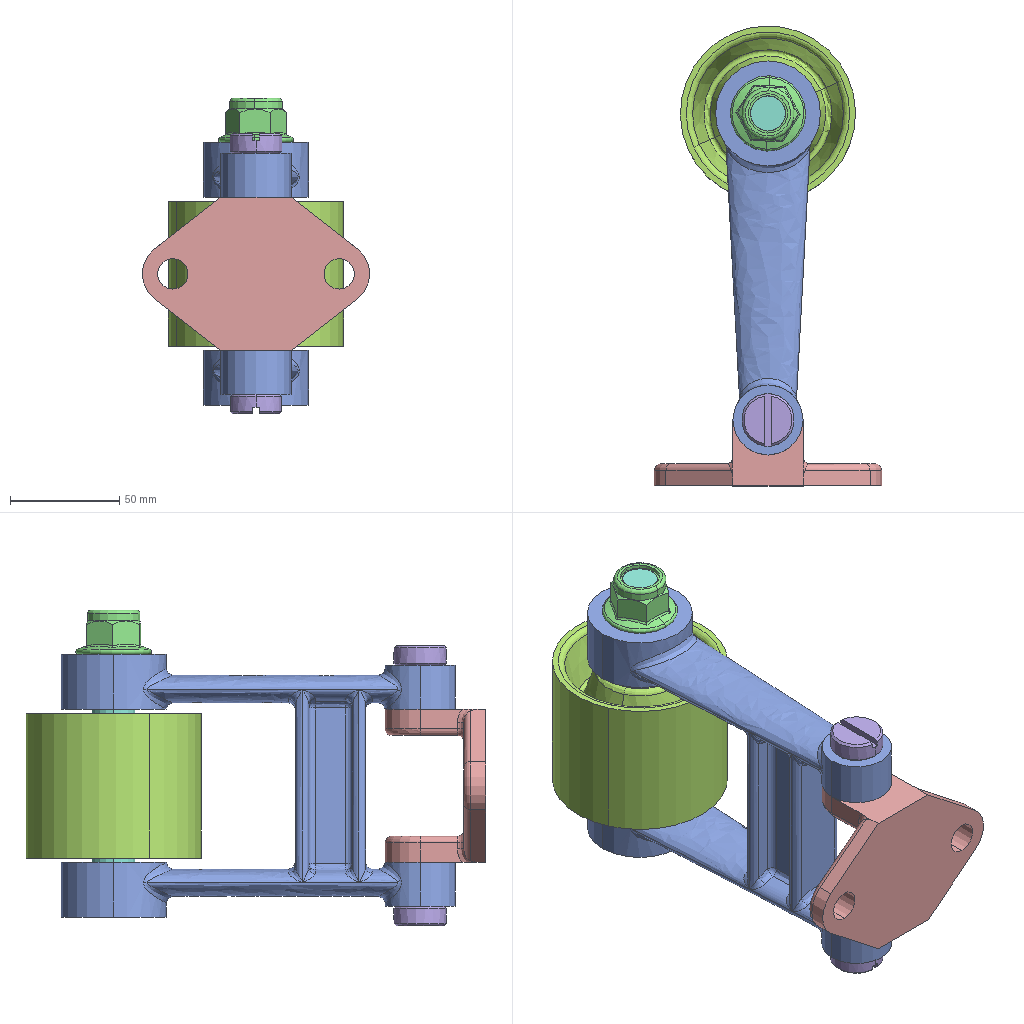Assembly | SolidWorks | 8 different items | 9 placed | box 104 x 210 x 144 mm
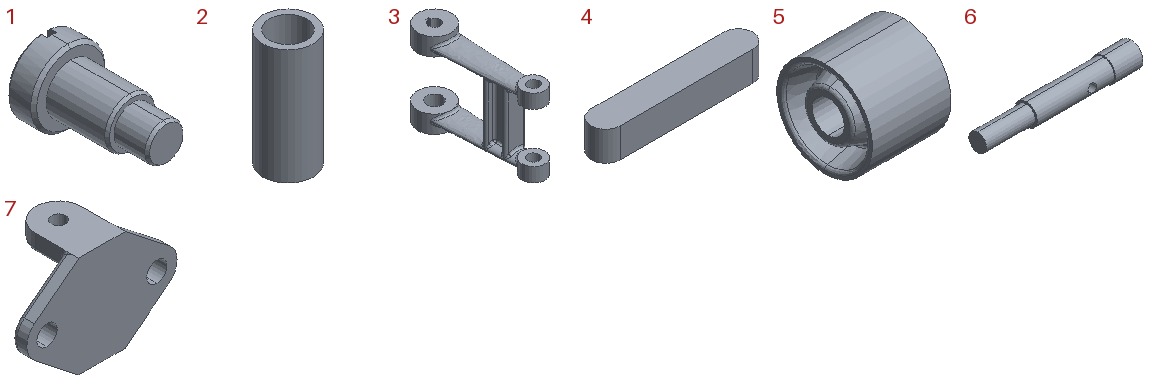Parts list (item | name | quantity | size | volume | features):
1 | - | x2 | 24 x 40 x 24 mm | 9026 mm3 | features Chamfer 2, ICE 1, Revolution 1
2 | - | x1 | 27 x 27 x 62 mm | 15842 mm3 | features Extrusion 1, ICE 1
3 | - | x1 | 48 x 180 x 120 mm | 202077 mm3 | features ICE 3, Blend 1, Extrusion 1, Fillet 1, MirrorSolid 1, Sculpt 1
4 | - | x1 | 22 x 4 x 4 mm | 338.265 mm3 | features Extrusion 1
5 | - | x1 | 66 x 80 x 80 mm | 217017 mm3 | features Revolution 1
6 | - | x1 | 139 x 22 x 22 mm | 37145 mm3 | features ICE 2, Revolution 1
7 | - | x1 | 104 x 46 x 70 mm | 71759 mm3 | features Fillet 3, Extrusion 1, ICE 1, MirrorPattern 1
8 | prevailing torque nut flange insert-2_din | x1 | - | - | -
Mates (type | each side: item.copy, entity, surface, feature):
Concentric | 7.1 face cylinder Mirror1 | 3.1 face cylinder Mirror2
Coincident | 7.1 edge | 3.1 edge
Concentric | 3.1 face cylinder Mirror2 | 5.1 face cylinder Revolve1
Width | 3.1 face plane Mirror2 | 3.1 face plane Boss-Extrude1 | 5.1 face plane Revolve1 | 5.1 face plane Revolve1
Concentric | 3.1 face cylinder Mirror2 | 2.1 face cylinder Boss-Extrude1
Concentric | 2.1 face cylinder Boss-Extrude1 | 6.1 face cylinder Revolve2
Concentric | 2.1 face cylinder Cut-Extrude1 | 6.1 face cylinder Cut-Extrude2
Coincident | 7.1 plane | 3.1 plane
Width | 5.1 face plane Revolve1 | 5.1 face plane Revolve1 | 2.1 face plane Boss-Extrude1 | 2.1 face plane Boss-Extrude1
Parallel | 3.1 face plane Boss-Extrude3 | 6.1 face plane Cut-Extrude1
Coincident | 6.1 edge | 4.1 edge
Coincident | 6.1 face plane Cut-Extrude1 | 4.1 face plane Boss-Extrude1
Concentric | 3.1 face cylinder Mirror2 | 1.1 face cylinder Revolve1
Coincident | 3.1 face plane Mirror2 | 1.1 face plane Revolve1
Coincident | 3.1 face cylinder Intersect1 | 1.2 edge
Coincident | 3.1 face plane Cut-Extrude1 | 1.2 face plane Revolve1